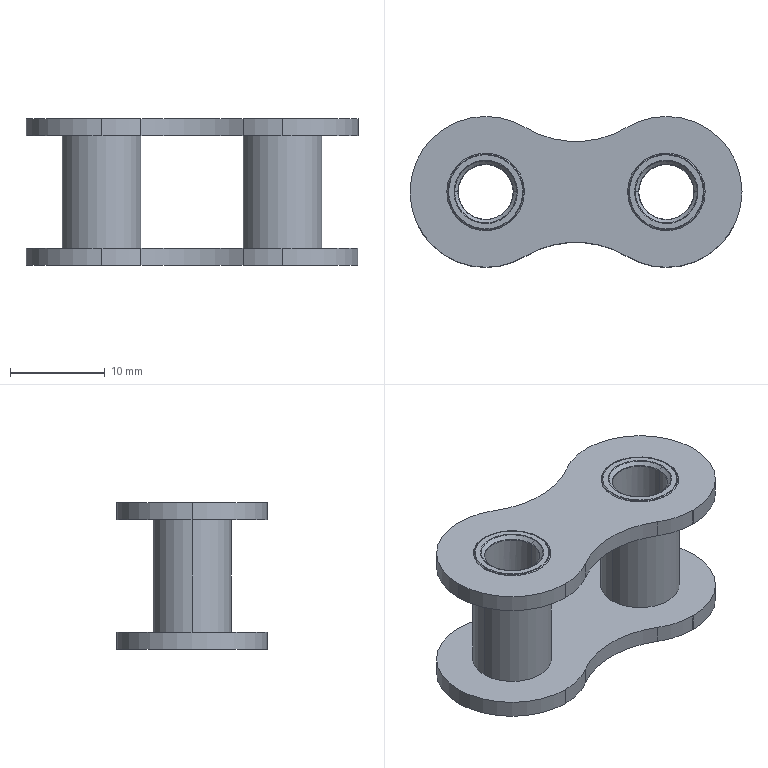Part | STEP file | 12b-1_02 | 1 solid | 92 faces | box 35 x 15.9 x 15.6 mm | volume 2056 mm3 | cylinder 34 | spline 24 | cone 18 | plane 16 | commonest cylinder face diameters 15.9 x14 8.18 x8 5.8 x4 8.29 x4 20.8 x4